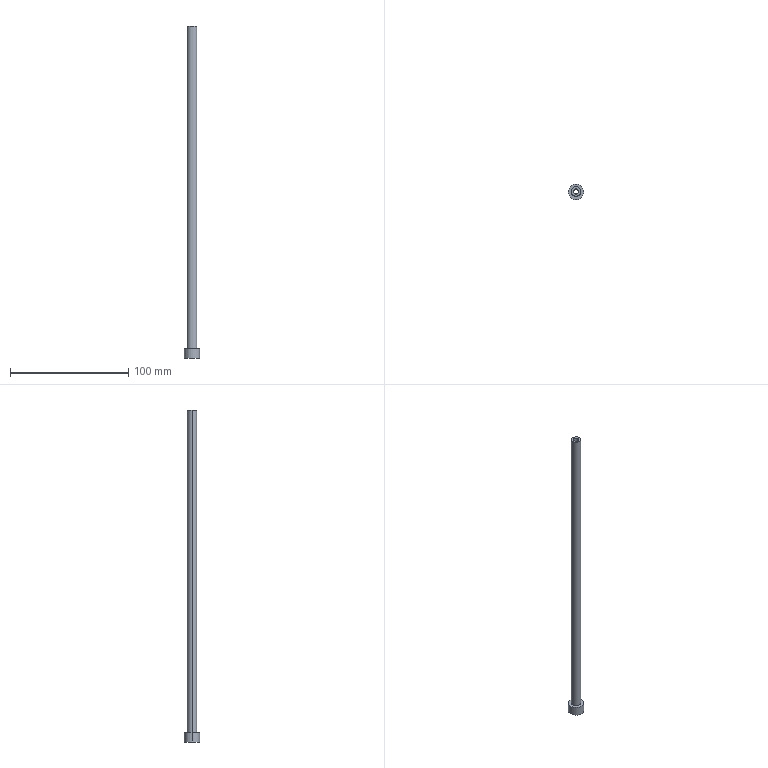Part | Creo | 1 solid | 9 faces | box 13 x 13 x 280.289 mm | volume 10291 mm3 | cylinder 6 | plane 3 | commonest cylinder face diameters 4.5 x2 8 x2 13 x2
STEP:
#1=CARTESIAN_POINT('',(77.346,-142.631,19.789));
#2=VERTEX_POINT('',#1);
#3=CARTESIAN_POINT('',(85.346,-142.631,19.789));
#4=VERTEX_POINT('',#3);
#5=CARTESIAN_POINT('',(81.346,-142.631,19.789));
#6=DIRECTION('',(0.,0.,1.));
#7=DIRECTION('',(-1.,0.,0.));
#8=AXIS2_PLACEMENT_3D('',#5,#6,#7);
#9=CIRCLE('',#8,4.);
#10=EDGE_CURVE('',#2,#4,#9,.T.);
#11=ORIENTED_EDGE('',*,*,#10,.F.);
#12=CARTESIAN_POINT('',(81.346,-142.631,19.789));
#13=DIRECTION('',(0.,0.,1.));
#14=DIRECTION('',(1.,0.,0.));
#15=AXIS2_PLACEMENT_3D('',#12,#13,#14);
#16=CIRCLE('',#15,4.);
#17=EDGE_CURVE('',#4,#2,#16,.T.);
#18=ORIENTED_EDGE('',*,*,#17,.F.);
#19=EDGE_LOOP('',(#11,#18));
#20=FACE_OUTER_BOUND('',#19,.F.);
#21=CARTESIAN_POINT('',(79.096,-142.631,19.789));
#22=VERTEX_POINT('',#21);
#23=CARTESIAN_POINT('',(83.596,-142.631,19.789));
#24=VERTEX_POINT('',#23);
#25=CARTESIAN_POINT('',(81.346,-142.631,19.789));
#26=DIRECTION('',(0.,0.,-1.));
#27=DIRECTION('',(-1.,0.,0.));
#28=AXIS2_PLACEMENT_3D('',#25,#26,#27);
#29=CIRCLE('',#28,2.25);
#30=EDGE_CURVE('',#22,#24,#29,.T.);
#31=ORIENTED_EDGE('',*,*,#30,.F.);
#32=CARTESIAN_POINT('',(81.346,-142.631,19.789));
#33=DIRECTION('',(0.,0.,-1.));
#34=DIRECTION('',(1.,0.,0.));
#35=AXIS2_PLACEMENT_3D('',#32,#33,#34);
#36=CIRCLE('',#35,2.25);
#37=EDGE_CURVE('',#24,#22,#36,.T.);
#38=ORIENTED_EDGE('',*,*,#37,.F.);
#39=EDGE_LOOP('',(#31,#38));
#40=FACE_BOUND('',#39,.F.);
#41=CARTESIAN_POINT('',(81.346,-142.631,19.789));
#42=DIRECTION('',(0.,0.,1.));
#43=DIRECTION('',(1.,0.,0.));
#44=AXIS2_PLACEMENT_3D('',#41,#42,#43);
#45=PLANE('',#44);
#46=ADVANCED_FACE('',(#20,#40),#45,.T.);
#47=CARTESIAN_POINT('',(85.346,-142.631,-252.5));
#48=VERTEX_POINT('',#47);
#49=CARTESIAN_POINT('',(77.346,-142.631,-252.5));
#50=VERTEX_POINT('',#49);
#51=CARTESIAN_POINT('',(81.346,-142.631,-252.5));
#52=DIRECTION('',(0.,0.,-1.));
#53=DIRECTION('',(1.,0.,0.));
#54=AXIS2_PLACEMENT_3D('',#51,#52,#53);
#55=CIRCLE('',#54,4.);
#56=EDGE_CURVE('',#48,#50,#55,.T.);
#57=ORIENTED_EDGE('',*,*,#56,.T.);
#58=CARTESIAN_POINT('',(77.346,-142.631,-252.5));
#59=DIRECTION('',(0.,0.,1.));
#60=VECTOR('',#59,272.289);
#61=LINE('',#58,#60);
#62=EDGE_CURVE('',#50,#2,#61,.T.);
#63=ORIENTED_EDGE('',*,*,#62,.T.);
#64=ORIENTED_EDGE('',*,*,#10,.T.);
#65=CARTESIAN_POINT('',(85.346,-142.631,-252.5));
#66=DIRECTION('',(0.,0.,1.));
#67=VECTOR('',#66,272.289);
#68=LINE('',#65,#67);
#69=EDGE_CURVE('',#48,#4,#68,.T.);
#70=ORIENTED_EDGE('',*,*,#69,.F.);
#71=EDGE_LOOP('',(#57,#63,#64,#70));
#72=FACE_OUTER_BOUND('',#71,.F.);
#73=CARTESIAN_POINT('',(81.346,-142.631,-255.5));
#74=DIRECTION('',(0.,0.,1.));
#75=DIRECTION('',(1.,0.,0.));
#76=AXIS2_PLACEMENT_3D('',#73,#74,#75);
#77=CYLINDRICAL_SURFACE('',#76,4.);
#78=ADVANCED_FACE('',(#72),#77,.T.);
#79=CARTESIAN_POINT('',(74.846,-142.631,-252.5));
#80=VERTEX_POINT('',#79);
#81=CARTESIAN_POINT('',(87.846,-142.631,-252.5));
#82=VERTEX_POINT('',#81);
#83=CARTESIAN_POINT('',(81.346,-142.631,-252.5));
#84=DIRECTION('',(0.,0.,1.));
#85=DIRECTION('',(-1.,0.,0.));
#86=AXIS2_PLACEMENT_3D('',#83,#84,#85);
#87=CIRCLE('',#86,6.5);
#88=EDGE_CURVE('',#80,#82,#87,.T.);
#89=ORIENTED_EDGE('',*,*,#88,.F.);
#90=CARTESIAN_POINT('',(81.346,-142.631,-252.5));
#91=DIRECTION('',(0.,0.,1.));
#92=DIRECTION('',(1.,0.,0.));
#93=AXIS2_PLACEMENT_3D('',#90,#91,#92);
#94=CIRCLE('',#93,6.5);
#95=EDGE_CURVE('',#82,#80,#94,.T.);
#96=ORIENTED_EDGE('',*,*,#95,.F.);
#97=EDGE_LOOP('',(#89,#96));
#98=FACE_OUTER_BOUND('',#97,.F.);
#99=ORIENTED_EDGE('',*,*,#56,.F.);
#100=CARTESIAN_POINT('',(81.346,-142.631,-252.5));
#101=DIRECTION('',(0.,0.,-1.));
#102=DIRECTION('',(-1.,0.,0.));
#103=AXIS2_PLACEMENT_3D('',#100,#101,#102);
#104=CIRCLE('',#103,4.);
#105=EDGE_CURVE('',#50,#48,#104,.T.);
#106=ORIENTED_EDGE('',*,*,#105,.F.);
#107=EDGE_LOOP('',(#99,#106));
#108=FACE_BOUND('',#107,.F.);
#109=CARTESIAN_POINT('',(81.346,-142.631,-252.5));
#110=DIRECTION('',(0.,0.,1.));
#111=DIRECTION('',(1.,0.,0.));
#112=AXIS2_PLACEMENT_3D('',#109,#110,#111);
#113=PLANE('',#112);
#114=ADVANCED_FACE('',(#98,#108),#113,.T.);
#115=ORIENTED_EDGE('',*,*,#105,.T.);
#116=ORIENTED_EDGE('',*,*,#69,.T.);
#117=ORIENTED_EDGE('',*,*,#17,.T.);
#118=ORIENTED_EDGE('',*,*,#62,.F.);
#119=EDGE_LOOP('',(#115,#116,#117,#118));
#120=FACE_OUTER_BOUND('',#119,.F.);
#121=CARTESIAN_POINT('',(81.346,-142.631,-255.5));
#122=DIRECTION('',(0.,0.,1.));
#123=DIRECTION('',(1.,0.,0.));
#124=AXIS2_PLACEMENT_3D('',#121,#122,#123);
#125=CYLINDRICAL_SURFACE('',#124,4.);
#126=ADVANCED_FACE('',(#120),#125,.T.);
#127=ORIENTED_EDGE('',*,*,#88,.T.);
#128=CARTESIAN_POINT('',(87.846,-142.631,-260.5));
#129=VERTEX_POINT('',#128);
#130=CARTESIAN_POINT('',(87.846,-142.631,-260.5));
#131=DIRECTION('',(0.,0.,1.));
#132=VECTOR('',#131,8.);
#133=LINE('',#130,#132);
#134=EDGE_CURVE('',#129,#82,#133,.T.);
#135=ORIENTED_EDGE('',*,*,#134,.F.);
#136=CARTESIAN_POINT('',(74.846,-142.631,-260.5));
#137=VERTEX_POINT('',#136);
#138=CARTESIAN_POINT('',(81.346,-142.631,-260.5));
#139=DIRECTION('',(0.,0.,-1.));
#140=DIRECTION('',(1.,0.,0.));
#141=AXIS2_PLACEMENT_3D('',#138,#139,#140);
#142=CIRCLE('',#141,6.5);
#143=EDGE_CURVE('',#129,#137,#142,.T.);
#144=ORIENTED_EDGE('',*,*,#143,.T.);
#145=CARTESIAN_POINT('',(74.846,-142.631,-260.5));
#146=DIRECTION('',(0.,0.,1.));
#147=VECTOR('',#146,8.);
#148=LINE('',#145,#147);
#149=EDGE_CURVE('',#137,#80,#148,.T.);
#150=ORIENTED_EDGE('',*,*,#149,.T.);
#151=EDGE_LOOP('',(#127,#135,#144,#150));
#152=FACE_OUTER_BOUND('',#151,.F.);
#153=CARTESIAN_POINT('',(81.346,-142.631,-260.5));
#154=DIRECTION('',(0.,0.,1.));
#155=DIRECTION('',(1.,0.,0.));
#156=AXIS2_PLACEMENT_3D('',#153,#154,#155);
#157=CYLINDRICAL_SURFACE('',#156,6.5);
#158=ADVANCED_FACE('',(#152),#157,.T.);
#159=ORIENTED_EDGE('',*,*,#95,.T.);
#160=ORIENTED_EDGE('',*,*,#149,.F.);
#161=CARTESIAN_POINT('',(81.346,-142.631,-260.5));
#162=DIRECTION('',(0.,0.,-1.));
#163=DIRECTION('',(-1.,0.,0.));
#164=AXIS2_PLACEMENT_3D('',#161,#162,#163);
#165=CIRCLE('',#164,6.5);
#166=EDGE_CURVE('',#137,#129,#165,.T.);
#167=ORIENTED_EDGE('',*,*,#166,.T.);
#168=ORIENTED_EDGE('',*,*,#134,.T.);
#169=EDGE_LOOP('',(#159,#160,#167,#168));
#170=FACE_OUTER_BOUND('',#169,.F.);
#171=CARTESIAN_POINT('',(81.346,-142.631,-260.5));
#172=DIRECTION('',(0.,0.,1.));
#173=DIRECTION('',(1.,0.,0.));
#174=AXIS2_PLACEMENT_3D('',#171,#172,#173);
#175=CYLINDRICAL_SURFACE('',#174,6.5);
#176=ADVANCED_FACE('',(#170),#175,.T.);
#177=ORIENTED_EDGE('',*,*,#143,.F.);
#178=ORIENTED_EDGE('',*,*,#166,.F.);
#179=EDGE_LOOP('',(#177,#178));
#180=FACE_OUTER_BOUND('',#179,.F.);
#181=CARTESIAN_POINT('',(83.596,-142.631,-260.5));
#182=VERTEX_POINT('',#181);
#183=CARTESIAN_POINT('',(79.096,-142.631,-260.5));
#184=VERTEX_POINT('',#183);
#185=CARTESIAN_POINT('',(81.346,-142.631,-260.5));
#186=DIRECTION('',(0.,0.,1.));
#187=DIRECTION('',(1.,0.,0.));
#188=AXIS2_PLACEMENT_3D('',#185,#186,#187);
#189=CIRCLE('',#188,2.25);
#190=EDGE_CURVE('',#182,#184,#189,.T.);
#191=ORIENTED_EDGE('',*,*,#190,.F.);
#192=CARTESIAN_POINT('',(81.346,-142.631,-260.5));
#193=DIRECTION('',(0.,0.,1.));
#194=DIRECTION('',(-1.,0.,0.));
#195=AXIS2_PLACEMENT_3D('',#192,#193,#194);
#196=CIRCLE('',#195,2.25);
#197=EDGE_CURVE('',#184,#182,#196,.T.);
#198=ORIENTED_EDGE('',*,*,#197,.F.);
#199=EDGE_LOOP('',(#191,#198));
#200=FACE_BOUND('',#199,.F.);
#201=CARTESIAN_POINT('',(81.346,-142.631,-260.5));
#202=DIRECTION('',(0.,0.,-1.));
#203=DIRECTION('',(-1.,0.,0.));
#204=AXIS2_PLACEMENT_3D('',#201,#202,#203);
#205=PLANE('',#204);
#206=ADVANCED_FACE('',(#180,#200),#205,.T.);
#207=ORIENTED_EDGE('',*,*,#30,.T.);
#208=CARTESIAN_POINT('',(83.596,-142.631,-260.5));
#209=DIRECTION('',(0.,0.,1.));
#210=VECTOR('',#209,280.289);
#211=LINE('',#208,#210);
#212=EDGE_CURVE('',#182,#24,#211,.T.);
#213=ORIENTED_EDGE('',*,*,#212,.F.);
#214=ORIENTED_EDGE('',*,*,#190,.T.);
#215=CARTESIAN_POINT('',(79.096,-142.631,-260.5));
#216=DIRECTION('',(0.,0.,1.));
#217=VECTOR('',#216,280.289);
#218=LINE('',#215,#217);
#219=EDGE_CURVE('',#184,#22,#218,.T.);
#220=ORIENTED_EDGE('',*,*,#219,.T.);
#221=EDGE_LOOP('',(#207,#213,#214,#220));
#222=FACE_OUTER_BOUND('',#221,.F.);
#223=CARTESIAN_POINT('',(81.346,-142.631,-255.5));
#224=DIRECTION('',(0.,0.,1.));
#225=DIRECTION('',(1.,0.,0.));
#226=AXIS2_PLACEMENT_3D('',#223,#224,#225);
#227=CYLINDRICAL_SURFACE('',#226,2.25);
#228=ADVANCED_FACE('',(#222),#227,.F.);
#229=ORIENTED_EDGE('',*,*,#37,.T.);
#230=ORIENTED_EDGE('',*,*,#219,.F.);
#231=ORIENTED_EDGE('',*,*,#197,.T.);
#232=ORIENTED_EDGE('',*,*,#212,.T.);
#233=EDGE_LOOP('',(#229,#230,#231,#232));
#234=FACE_OUTER_BOUND('',#233,.F.);
#235=CARTESIAN_POINT('',(81.346,-142.631,-255.5));
#236=DIRECTION('',(0.,0.,1.));
#237=DIRECTION('',(1.,0.,0.));
#238=AXIS2_PLACEMENT_3D('',#235,#236,#237);
#239=CYLINDRICAL_SURFACE('',#238,2.25);
#240=ADVANCED_FACE('',(#234),#239,.F.);
#241=CLOSED_SHELL('',(#46,#78,#114,#126,#158,#176,#206,#228,#240));
#242=MANIFOLD_SOLID_BREP('',#241);
#243=(LENGTH_UNIT()NAMED_UNIT(*)SI_UNIT(.MILLI.,.METRE.));
#244=UNCERTAINTY_MEASURE_WITH_UNIT(LENGTH_MEASURE(0.02809),#243,'','');
#245=(NAMED_UNIT(*)PLANE_ANGLE_UNIT()SI_UNIT($,.RADIAN.));
#246=PLANE_ANGLE_MEASURE_WITH_UNIT(PLANE_ANGLE_MEASURE(0.01745),#245);
#247=(CONVERSION_BASED_UNIT('DEGREE',#246)NAMED_UNIT(*)PLANE_ANGLE_UNIT());
#248=(NAMED_UNIT(*)SI_UNIT($,.STERADIAN.)SOLID_ANGLE_UNIT());
#249=(GEOMETRIC_REPRESENTATION_CONTEXT(3)GLOBAL_UNCERTAINTY_ASSIGNED_CONTEXT((#244))GLOBAL_UNIT_ASSIGNED_CONTEXT((#243,#247,#248))REPRESENTATION_CONTEXT('',''));
#250=ADVANCED_BREP_SHAPE_REPRESENTATION('',(#242),#249);